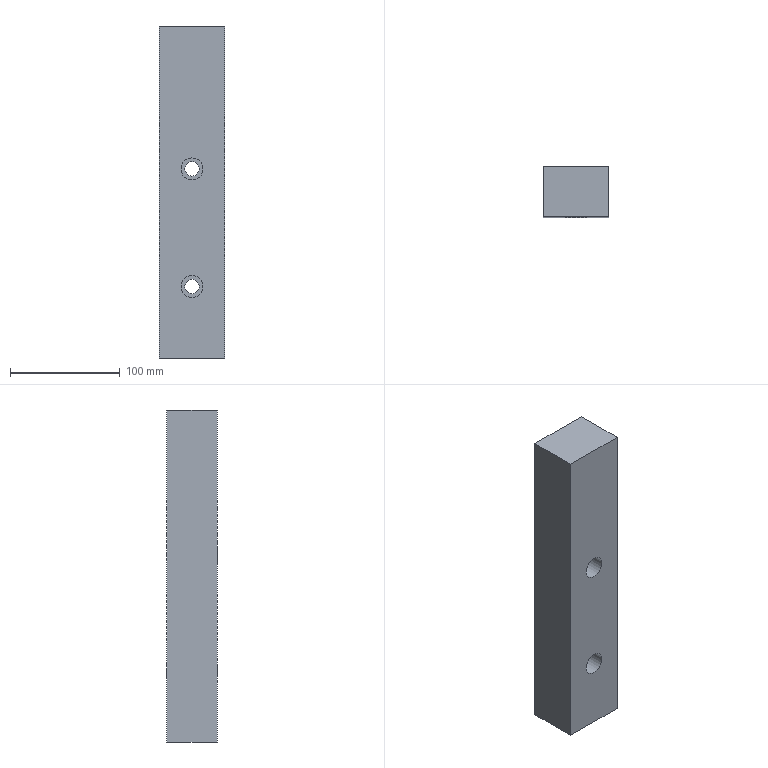Part | NX | features solid 2 | 1 solid | 12 faces | box 60 x 46 x 302 mm | volume 812237 mm3 | plane 8 | cylinder 4 | commonest cylinder face diameters 13 x2 20 x2
STEP:
#1=CARTESIAN_POINT('',(-307.074,-500.,253.));
#2=VERTEX_POINT('',#1);
#3=CARTESIAN_POINT('',(-307.074,-500.,243.));
#4=DIRECTION('',(0.,1.,0.));
#5=DIRECTION('',(0.,0.,1.));
#6=AXIS2_PLACEMENT_3D('',#3,#4,#5);
#7=CIRCLE('',#6,10.);
#8=EDGE_CURVE('',#2,#2,#7,.T.);
#9=ORIENTED_EDGE('',*,*,#8,.T.);
#10=EDGE_LOOP('',(#9));
#11=FACE_BOUND('',#10,.T.);
#12=CARTESIAN_POINT('',(-307.074,-500.,360.));
#13=VERTEX_POINT('',#12);
#14=CARTESIAN_POINT('',(-307.074,-500.,350.));
#15=DIRECTION('',(0.,1.,0.));
#16=DIRECTION('',(0.,0.,1.));
#17=AXIS2_PLACEMENT_3D('',#14,#15,#16);
#18=CIRCLE('',#17,10.);
#19=EDGE_CURVE('',#13,#13,#18,.T.);
#20=ORIENTED_EDGE('',*,*,#19,.T.);
#21=EDGE_LOOP('',(#20));
#22=FACE_BOUND('',#21,.T.);
#23=CARTESIAN_POINT('',(-277.074,-500.,480.));
#24=VERTEX_POINT('',#23);
#25=CARTESIAN_POINT('',(-337.074,-500.,480.));
#26=VERTEX_POINT('',#25);
#27=CARTESIAN_POINT('',(-277.074,-500.,480.));
#28=DIRECTION('',(1.,0.,0.));
#29=VECTOR('',#28,1000.);
#30=LINE('',#27,#29);
#31=EDGE_CURVE('',#24,#26,#30,.F.);
#32=ORIENTED_EDGE('',*,*,#31,.T.);
#33=CARTESIAN_POINT('',(-337.074,-500.,178.));
#34=VERTEX_POINT('',#33);
#35=CARTESIAN_POINT('',(-337.074,-500.,487.6));
#36=DIRECTION('',(0.,0.,-1.));
#37=VECTOR('',#36,1000.);
#38=LINE('',#35,#37);
#39=EDGE_CURVE('',#34,#26,#38,.F.);
#40=ORIENTED_EDGE('',*,*,#39,.F.);
#41=CARTESIAN_POINT('',(-277.074,-500.,178.));
#42=VERTEX_POINT('',#41);
#43=CARTESIAN_POINT('',(-277.074,-500.,178.));
#44=DIRECTION('',(-1.,0.,0.));
#45=VECTOR('',#44,1000.);
#46=LINE('',#43,#45);
#47=EDGE_CURVE('',#42,#34,#46,.T.);
#48=ORIENTED_EDGE('',*,*,#47,.F.);
#49=CARTESIAN_POINT('',(-277.074,-500.,192.6));
#50=DIRECTION('',(0.,0.,1.));
#51=VECTOR('',#50,1000.);
#52=LINE('',#49,#51);
#53=EDGE_CURVE('',#42,#24,#52,.T.);
#54=ORIENTED_EDGE('',*,*,#53,.T.);
#55=EDGE_LOOP('',(#32,#40,#48,#54));
#56=FACE_BOUND('',#55,.T.);
#57=CARTESIAN_POINT('',(-277.074,-500.,192.6));
#58=DIRECTION('',(0.,1.,0.));
#59=DIRECTION('',(0.,0.,1.));
#60=AXIS2_PLACEMENT_3D('',#57,#58,#59);
#61=PLANE('',#60);
#62=ADVANCED_FACE('',(#11,#22,#56),#61,.F.);
#63=CARTESIAN_POINT('',(-337.074,-454.,480.));
#64=VERTEX_POINT('',#63);
#65=CARTESIAN_POINT('',(-337.074,-457.004,480.));
#66=DIRECTION('',(0.,1.,0.));
#67=VECTOR('',#66,1000.);
#68=LINE('',#65,#67);
#69=EDGE_CURVE('',#26,#64,#68,.T.);
#70=ORIENTED_EDGE('',*,*,#69,.T.);
#71=CARTESIAN_POINT('',(-337.074,-454.,178.));
#72=VERTEX_POINT('',#71);
#73=CARTESIAN_POINT('',(-337.074,-454.,192.6));
#74=DIRECTION('',(0.,0.,-1.));
#75=VECTOR('',#74,1000.);
#76=LINE('',#73,#75);
#77=EDGE_CURVE('',#72,#64,#76,.F.);
#78=ORIENTED_EDGE('',*,*,#77,.F.);
#79=CARTESIAN_POINT('',(-337.074,-457.004,178.));
#80=DIRECTION('',(0.,-1.,0.));
#81=VECTOR('',#80,1000.);
#82=LINE('',#79,#81);
#83=EDGE_CURVE('',#34,#72,#82,.F.);
#84=ORIENTED_EDGE('',*,*,#83,.F.);
#85=ORIENTED_EDGE('',*,*,#39,.T.);
#86=EDGE_LOOP('',(#70,#78,#84,#85));
#87=FACE_BOUND('',#86,.T.);
#88=CARTESIAN_POINT('',(-337.074,-457.004,487.6));
#89=DIRECTION('',(-1.,0.,0.));
#90=DIRECTION('',(0.,0.,-1.));
#91=AXIS2_PLACEMENT_3D('',#88,#89,#90);
#92=PLANE('',#91);
#93=ADVANCED_FACE('',(#87),#92,.T.);
#94=CARTESIAN_POINT('',(-307.074,-454.,236.5));
#95=VERTEX_POINT('',#94);
#96=CARTESIAN_POINT('',(-307.074,-454.,243.));
#97=DIRECTION('',(0.,-1.,0.));
#98=DIRECTION('',(0.,0.,-1.));
#99=AXIS2_PLACEMENT_3D('',#96,#97,#98);
#100=CIRCLE('',#99,6.5);
#101=EDGE_CURVE('',#95,#95,#100,.T.);
#102=ORIENTED_EDGE('',*,*,#101,.T.);
#103=EDGE_LOOP('',(#102));
#104=FACE_BOUND('',#103,.T.);
#105=CARTESIAN_POINT('',(-307.074,-454.,343.5));
#106=VERTEX_POINT('',#105);
#107=CARTESIAN_POINT('',(-307.074,-454.,350.));
#108=DIRECTION('',(0.,-1.,0.));
#109=DIRECTION('',(0.,0.,-1.));
#110=AXIS2_PLACEMENT_3D('',#107,#108,#109);
#111=CIRCLE('',#110,6.5);
#112=EDGE_CURVE('',#106,#106,#111,.T.);
#113=ORIENTED_EDGE('',*,*,#112,.T.);
#114=EDGE_LOOP('',(#113));
#115=FACE_BOUND('',#114,.T.);
#116=CARTESIAN_POINT('',(-277.074,-454.,480.));
#117=VERTEX_POINT('',#116);
#118=CARTESIAN_POINT('',(-337.074,-454.,480.));
#119=DIRECTION('',(-1.,0.,0.));
#120=VECTOR('',#119,1000.);
#121=LINE('',#118,#120);
#122=EDGE_CURVE('',#64,#117,#121,.F.);
#123=ORIENTED_EDGE('',*,*,#122,.T.);
#124=CARTESIAN_POINT('',(-277.074,-454.,178.));
#125=VERTEX_POINT('',#124);
#126=CARTESIAN_POINT('',(-277.074,-454.,192.6));
#127=DIRECTION('',(0.,0.,-1.));
#128=VECTOR('',#127,1000.);
#129=LINE('',#126,#128);
#130=EDGE_CURVE('',#117,#125,#129,.T.);
#131=ORIENTED_EDGE('',*,*,#130,.T.);
#132=CARTESIAN_POINT('',(-337.074,-454.,178.));
#133=DIRECTION('',(1.,0.,0.));
#134=VECTOR('',#133,1000.);
#135=LINE('',#132,#134);
#136=EDGE_CURVE('',#72,#125,#135,.T.);
#137=ORIENTED_EDGE('',*,*,#136,.F.);
#138=ORIENTED_EDGE('',*,*,#77,.T.);
#139=EDGE_LOOP('',(#123,#131,#137,#138));
#140=FACE_BOUND('',#139,.T.);
#141=CARTESIAN_POINT('',(-337.074,-454.,192.6));
#142=DIRECTION('',(0.,-1.,0.));
#143=DIRECTION('',(0.,0.,-1.));
#144=AXIS2_PLACEMENT_3D('',#141,#142,#143);
#145=PLANE('',#144);
#146=ADVANCED_FACE('',(#104,#115,#140),#145,.F.);
#147=ORIENTED_EDGE('',*,*,#130,.F.);
#148=CARTESIAN_POINT('',(-277.074,388.333,480.));
#149=DIRECTION('',(0.,-1.,0.));
#150=VECTOR('',#149,1000.);
#151=LINE('',#148,#150);
#152=EDGE_CURVE('',#24,#117,#151,.F.);
#153=ORIENTED_EDGE('',*,*,#152,.F.);
#154=ORIENTED_EDGE('',*,*,#53,.F.);
#155=CARTESIAN_POINT('',(-277.074,-512.004,178.));
#156=DIRECTION('',(0.,1.,0.));
#157=VECTOR('',#156,1000.);
#158=LINE('',#155,#157);
#159=EDGE_CURVE('',#42,#125,#158,.T.);
#160=ORIENTED_EDGE('',*,*,#159,.T.);
#161=EDGE_LOOP('',(#147,#153,#154,#160));
#162=FACE_BOUND('',#161,.T.);
#163=CARTESIAN_POINT('',(-277.074,-457.004,487.6));
#164=DIRECTION('',(-1.,0.,0.));
#165=DIRECTION('',(0.,0.,-1.));
#166=AXIS2_PLACEMENT_3D('',#163,#164,#165);
#167=PLANE('',#166);
#168=ADVANCED_FACE('',(#162),#167,.F.);
#169=ORIENTED_EDGE('',*,*,#136,.T.);
#170=ORIENTED_EDGE('',*,*,#159,.F.);
#171=ORIENTED_EDGE('',*,*,#47,.T.);
#172=ORIENTED_EDGE('',*,*,#83,.T.);
#173=EDGE_LOOP('',(#169,#170,#171,#172));
#174=FACE_BOUND('',#173,.T.);
#175=CARTESIAN_POINT('',(-337.074,-512.004,178.));
#176=DIRECTION('',(0.,0.,-1.));
#177=DIRECTION('',(0.,1.,0.));
#178=AXIS2_PLACEMENT_3D('',#175,#176,#177);
#179=PLANE('',#178);
#180=ADVANCED_FACE('',(#174),#179,.T.);
#181=ORIENTED_EDGE('',*,*,#152,.T.);
#182=ORIENTED_EDGE('',*,*,#122,.F.);
#183=ORIENTED_EDGE('',*,*,#69,.F.);
#184=ORIENTED_EDGE('',*,*,#31,.F.);
#185=EDGE_LOOP('',(#181,#182,#183,#184));
#186=FACE_BOUND('',#185,.T.);
#187=CARTESIAN_POINT('',(238.333,388.333,480.));
#188=DIRECTION('',(0.,0.,1.));
#189=DIRECTION('',(0.,-1.,0.));
#190=AXIS2_PLACEMENT_3D('',#187,#188,#189);
#191=PLANE('',#190);
#192=ADVANCED_FACE('',(#186),#191,.T.);
#193=CARTESIAN_POINT('',(-307.074,-475.,340.));
#194=VERTEX_POINT('',#193);
#195=CARTESIAN_POINT('',(-307.074,-475.,350.));
#196=DIRECTION('',(0.,-1.,0.));
#197=DIRECTION('',(0.,0.,-1.));
#198=AXIS2_PLACEMENT_3D('',#195,#196,#197);
#199=CIRCLE('',#198,10.);
#200=EDGE_CURVE('',#194,#194,#199,.T.);
#201=ORIENTED_EDGE('',*,*,#200,.F.);
#202=EDGE_LOOP('',(#201));
#203=FACE_BOUND('',#202,.T.);
#204=ORIENTED_EDGE('',*,*,#19,.F.);
#205=EDGE_LOOP('',(#204));
#206=FACE_BOUND('',#205,.T.);
#207=CARTESIAN_POINT('',(-307.074,-475.,350.));
#208=DIRECTION('',(0.,-1.,0.));
#209=DIRECTION('',(0.,0.,-1.));
#210=AXIS2_PLACEMENT_3D('',#207,#208,#209);
#211=CYLINDRICAL_SURFACE('',#210,10.);
#212=ADVANCED_FACE('',(#203,#206),#211,.F.);
#213=CARTESIAN_POINT('',(-307.074,-475.,356.5));
#214=VERTEX_POINT('',#213);
#215=CARTESIAN_POINT('',(-307.074,-475.,350.));
#216=DIRECTION('',(0.,1.,0.));
#217=DIRECTION('',(0.,0.,1.));
#218=AXIS2_PLACEMENT_3D('',#215,#216,#217);
#219=CIRCLE('',#218,6.5);
#220=EDGE_CURVE('',#214,#214,#219,.F.);
#221=ORIENTED_EDGE('',*,*,#220,.T.);
#222=EDGE_LOOP('',(#221));
#223=FACE_BOUND('',#222,.T.);
#224=ORIENTED_EDGE('',*,*,#112,.F.);
#225=EDGE_LOOP('',(#224));
#226=FACE_BOUND('',#225,.T.);
#227=CARTESIAN_POINT('',(-307.074,-435.,350.));
#228=DIRECTION('',(0.,-1.,0.));
#229=DIRECTION('',(0.,0.,-1.));
#230=AXIS2_PLACEMENT_3D('',#227,#228,#229);
#231=CYLINDRICAL_SURFACE('',#230,6.5);
#232=ADVANCED_FACE('',(#223,#226),#231,.F.);
#233=ORIENTED_EDGE('',*,*,#220,.F.);
#234=EDGE_LOOP('',(#233));
#235=FACE_BOUND('',#234,.T.);
#236=ORIENTED_EDGE('',*,*,#200,.T.);
#237=EDGE_LOOP('',(#236));
#238=FACE_BOUND('',#237,.T.);
#239=CARTESIAN_POINT('',(-307.074,-475.,350.));
#240=DIRECTION('',(0.,1.,0.));
#241=DIRECTION('',(0.,0.,1.));
#242=AXIS2_PLACEMENT_3D('',#239,#240,#241);
#243=PLANE('',#242);
#244=ADVANCED_FACE('',(#235,#238),#243,.F.);
#245=CARTESIAN_POINT('',(-307.074,-475.,233.));
#246=VERTEX_POINT('',#245);
#247=CARTESIAN_POINT('',(-307.074,-475.,243.));
#248=DIRECTION('',(0.,-1.,0.));
#249=DIRECTION('',(0.,0.,-1.));
#250=AXIS2_PLACEMENT_3D('',#247,#248,#249);
#251=CIRCLE('',#250,10.);
#252=EDGE_CURVE('',#246,#246,#251,.T.);
#253=ORIENTED_EDGE('',*,*,#252,.F.);
#254=EDGE_LOOP('',(#253));
#255=FACE_BOUND('',#254,.T.);
#256=ORIENTED_EDGE('',*,*,#8,.F.);
#257=EDGE_LOOP('',(#256));
#258=FACE_BOUND('',#257,.T.);
#259=CARTESIAN_POINT('',(-307.074,-475.,243.));
#260=DIRECTION('',(0.,-1.,0.));
#261=DIRECTION('',(0.,0.,-1.));
#262=AXIS2_PLACEMENT_3D('',#259,#260,#261);
#263=CYLINDRICAL_SURFACE('',#262,10.);
#264=ADVANCED_FACE('',(#255,#258),#263,.F.);
#265=CARTESIAN_POINT('',(-307.074,-475.,249.5));
#266=VERTEX_POINT('',#265);
#267=CARTESIAN_POINT('',(-307.074,-475.,243.));
#268=DIRECTION('',(0.,1.,0.));
#269=DIRECTION('',(0.,0.,1.));
#270=AXIS2_PLACEMENT_3D('',#267,#268,#269);
#271=CIRCLE('',#270,6.5);
#272=EDGE_CURVE('',#266,#266,#271,.F.);
#273=ORIENTED_EDGE('',*,*,#272,.T.);
#274=EDGE_LOOP('',(#273));
#275=FACE_BOUND('',#274,.T.);
#276=ORIENTED_EDGE('',*,*,#101,.F.);
#277=EDGE_LOOP('',(#276));
#278=FACE_BOUND('',#277,.T.);
#279=CARTESIAN_POINT('',(-307.074,-435.,243.));
#280=DIRECTION('',(0.,-1.,0.));
#281=DIRECTION('',(0.,0.,-1.));
#282=AXIS2_PLACEMENT_3D('',#279,#280,#281);
#283=CYLINDRICAL_SURFACE('',#282,6.5);
#284=ADVANCED_FACE('',(#275,#278),#283,.F.);
#285=ORIENTED_EDGE('',*,*,#272,.F.);
#286=EDGE_LOOP('',(#285));
#287=FACE_BOUND('',#286,.T.);
#288=ORIENTED_EDGE('',*,*,#252,.T.);
#289=EDGE_LOOP('',(#288));
#290=FACE_BOUND('',#289,.T.);
#291=CARTESIAN_POINT('',(-307.074,-475.,243.));
#292=DIRECTION('',(0.,1.,0.));
#293=DIRECTION('',(0.,0.,1.));
#294=AXIS2_PLACEMENT_3D('',#291,#292,#293);
#295=PLANE('',#294);
#296=ADVANCED_FACE('',(#287,#290),#295,.F.);
#297=CLOSED_SHELL('',(#62,#93,#146,#168,#180,#192,#212,#232,#244,#264,#284,#296));
#298=MANIFOLD_SOLID_BREP('',#297);
#299=(LENGTH_UNIT()NAMED_UNIT(*)SI_UNIT(.MILLI.,.METRE.));
#300=UNCERTAINTY_MEASURE_WITH_UNIT(LENGTH_MEASURE(0.00001),#299,'','');
#301=(NAMED_UNIT(*)PLANE_ANGLE_UNIT()SI_UNIT($,.RADIAN.));
#302=(NAMED_UNIT(*)SI_UNIT($,.STERADIAN.)SOLID_ANGLE_UNIT());
#303=(GEOMETRIC_REPRESENTATION_CONTEXT(3)GLOBAL_UNCERTAINTY_ASSIGNED_CONTEXT((#300))GLOBAL_UNIT_ASSIGNED_CONTEXT((#299,#301,#302))REPRESENTATION_CONTEXT('',''));
#304=ADVANCED_BREP_SHAPE_REPRESENTATION('',(#298),#303);